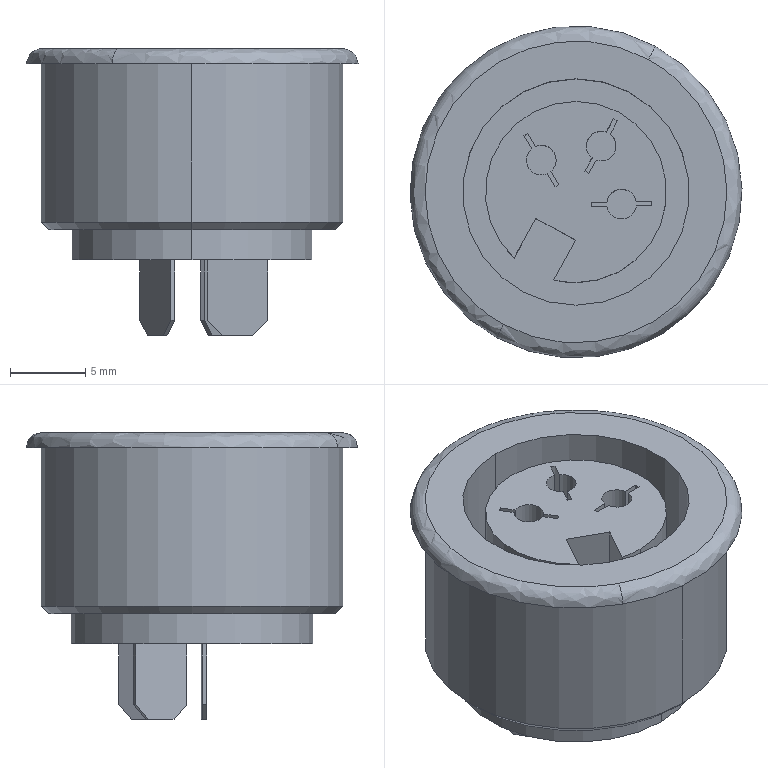Part | SolidWorks | features BaseBody 1 | 1 solid | 73 faces | box 22 x 22 x 19 mm | volume 3468 mm3 | plane 51 | cylinder 18 | spline 2 | cone 2 | commonest cylinder face diameters 1.972 x9 12 x3 15 x2 16 x2 20 x2